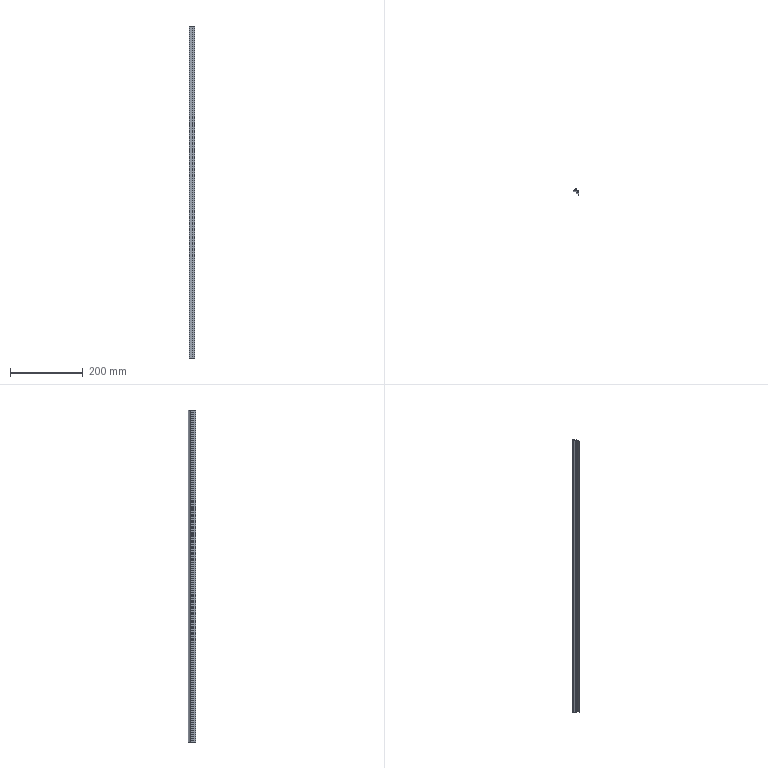Part | SolidWorks | features BaseBody 1, ICE 1, MoveFace 1 | 1 solid | 27 faces | box 14 x 20.3 x 914 mm | volume 46537 mm3 | plane 20 | cylinder 7 | commonest cylinder face diameters 0.387 x2 0.8 x2 0.4 x1 20 x1 22 x1
STEP:
#1=CARTESIAN_POINT('',(-5.304,-0.625,200.));
#2=VERTEX_POINT('',#1);
#3=CARTESIAN_POINT('',(-5.449,-0.8125,200.));
#4=VERTEX_POINT('',#3);
#5=CARTESIAN_POINT('',(-5.255,-0.8125,200.));
#6=DIRECTION('',(0.,0.,1.));
#7=DIRECTION('',(-1.,0.,0.));
#8=AXIS2_PLACEMENT_3D('',#5,#6,#7);
#9=CIRCLE('',#8,0.1937);
#10=EDGE_CURVE('',#2,#4,#9,.T.);
#11=ORIENTED_EDGE('',*,*,#10,.T.);
#12=CARTESIAN_POINT('',(-5.449,-0.8125,-714.));
#13=VERTEX_POINT('',#12);
#14=CARTESIAN_POINT('',(-5.449,-0.8125,230.));
#15=DIRECTION('',(0.,0.,-1.));
#16=VECTOR('',#15,1000.);
#17=LINE('',#14,#16);
#18=EDGE_CURVE('',#4,#13,#17,.T.);
#19=ORIENTED_EDGE('',*,*,#18,.T.);
#20=CARTESIAN_POINT('',(-5.304,-0.625,-714.));
#21=VERTEX_POINT('',#20);
#22=CARTESIAN_POINT('',(-5.255,-0.8125,-714.));
#23=DIRECTION('',(0.,0.,-1.));
#24=DIRECTION('',(1.,0.,0.));
#25=AXIS2_PLACEMENT_3D('',#22,#23,#24);
#26=CIRCLE('',#25,0.1937);
#27=EDGE_CURVE('',#13,#21,#26,.T.);
#28=ORIENTED_EDGE('',*,*,#27,.T.);
#29=CARTESIAN_POINT('',(-5.304,-0.625,230.));
#30=DIRECTION('',(0.,0.,-1.));
#31=VECTOR('',#30,1000.);
#32=LINE('',#29,#31);
#33=EDGE_CURVE('',#2,#21,#32,.T.);
#34=ORIENTED_EDGE('',*,*,#33,.F.);
#35=EDGE_LOOP('',(#11,#19,#28,#34));
#36=FACE_OUTER_BOUND('',#35,.T.);
#37=CARTESIAN_POINT('',(-5.255,-0.8125,230.));
#38=DIRECTION('',(0.,0.,-1.));
#39=DIRECTION('',(-1.,0.,0.));
#40=AXIS2_PLACEMENT_3D('',#37,#38,#39);
#41=CYLINDRICAL_SURFACE('',#40,0.1937);
#42=ADVANCED_FACE('',(#36),#41,.F.);
#43=CARTESIAN_POINT('',(5.,-1.,-714.));
#44=VERTEX_POINT('',#43);
#45=CARTESIAN_POINT('',(5.,-14.3,-714.));
#46=VERTEX_POINT('',#45);
#47=CARTESIAN_POINT('',(5.,29.623,-714.));
#48=DIRECTION('',(0.,-1.,0.));
#49=VECTOR('',#48,1000.);
#50=LINE('',#47,#49);
#51=EDGE_CURVE('',#44,#46,#50,.T.);
#52=ORIENTED_EDGE('',*,*,#51,.F.);
#53=CARTESIAN_POINT('',(5.,-1.,200.));
#54=VERTEX_POINT('',#53);
#55=CARTESIAN_POINT('',(5.,-1.,230.));
#56=DIRECTION('',(0.,0.,-1.));
#57=VECTOR('',#56,1000.);
#58=LINE('',#55,#57);
#59=EDGE_CURVE('',#54,#44,#58,.T.);
#60=ORIENTED_EDGE('',*,*,#59,.F.);
#61=CARTESIAN_POINT('',(5.,-14.3,200.));
#62=VERTEX_POINT('',#61);
#63=CARTESIAN_POINT('',(5.,-14.3,200.));
#64=DIRECTION('',(0.,1.,0.));
#65=VECTOR('',#64,1000.);
#66=LINE('',#63,#65);
#67=EDGE_CURVE('',#62,#54,#66,.T.);
#68=ORIENTED_EDGE('',*,*,#67,.F.);
#69=CARTESIAN_POINT('',(5.,-14.3,230.));
#70=DIRECTION('',(0.,0.,1.));
#71=VECTOR('',#70,1000.);
#72=LINE('',#69,#71);
#73=EDGE_CURVE('',#46,#62,#72,.T.);
#74=ORIENTED_EDGE('',*,*,#73,.F.);
#75=EDGE_LOOP('',(#52,#60,#68,#74));
#76=FACE_OUTER_BOUND('',#75,.T.);
#77=CARTESIAN_POINT('',(5.,-14.3,230.));
#78=DIRECTION('',(-1.,0.,0.));
#79=DIRECTION('',(0.,0.,1.));
#80=AXIS2_PLACEMENT_3D('',#77,#78,#79);
#81=PLANE('',#80);
#82=ADVANCED_FACE('',(#76),#81,.F.);
#83=CARTESIAN_POINT('',(-9.,-2.,-714.));
#84=VERTEX_POINT('',#83);
#85=CARTESIAN_POINT('',(-9.,-2.,200.));
#86=VERTEX_POINT('',#85);
#87=CARTESIAN_POINT('',(-9.,-2.,230.));
#88=DIRECTION('',(0.,0.,1.));
#89=VECTOR('',#88,1000.);
#90=LINE('',#87,#89);
#91=EDGE_CURVE('',#84,#86,#90,.T.);
#92=ORIENTED_EDGE('',*,*,#91,.F.);
#93=CARTESIAN_POINT('',(0.9,-2.,-714.));
#94=VERTEX_POINT('',#93);
#95=CARTESIAN_POINT('',(5.,-2.,-714.));
#96=DIRECTION('',(-1.,0.,0.));
#97=VECTOR('',#96,1000.);
#98=LINE('',#95,#97);
#99=EDGE_CURVE('',#94,#84,#98,.T.);
#100=ORIENTED_EDGE('',*,*,#99,.F.);
#101=CARTESIAN_POINT('',(0.9,-2.,200.));
#102=VERTEX_POINT('',#101);
#103=CARTESIAN_POINT('',(0.9,-2.,230.));
#104=DIRECTION('',(0.,0.,-1.));
#105=VECTOR('',#104,1000.);
#106=LINE('',#103,#105);
#107=EDGE_CURVE('',#102,#94,#106,.T.);
#108=ORIENTED_EDGE('',*,*,#107,.F.);
#109=CARTESIAN_POINT('',(5.,-2.,200.));
#110=DIRECTION('',(1.,0.,0.));
#111=VECTOR('',#110,1000.);
#112=LINE('',#109,#111);
#113=EDGE_CURVE('',#86,#102,#112,.T.);
#114=ORIENTED_EDGE('',*,*,#113,.F.);
#115=EDGE_LOOP('',(#92,#100,#108,#114));
#116=FACE_OUTER_BOUND('',#115,.T.);
#117=CARTESIAN_POINT('',(-9.,-2.,230.));
#118=DIRECTION('',(0.,1.,0.));
#119=DIRECTION('',(0.,0.,1.));
#120=AXIS2_PLACEMENT_3D('',#117,#118,#119);
#121=PLANE('',#120);
#122=ADVANCED_FACE('',(#116),#121,.F.);
#123=CARTESIAN_POINT('',(4.,-6.,200.));
#124=VERTEX_POINT('',#123);
#125=CARTESIAN_POINT('',(4.,-3.,200.));
#126=VERTEX_POINT('',#125);
#127=CARTESIAN_POINT('',(4.,29.623,200.));
#128=DIRECTION('',(0.,1.,0.));
#129=VECTOR('',#128,1000.);
#130=LINE('',#127,#129);
#131=EDGE_CURVE('',#124,#126,#130,.T.);
#132=ORIENTED_EDGE('',*,*,#131,.F.);
#133=CARTESIAN_POINT('',(1.,-6.,200.));
#134=VERTEX_POINT('',#133);
#135=CARTESIAN_POINT('',(5.,-6.,200.));
#136=DIRECTION('',(1.,0.,0.));
#137=VECTOR('',#136,1000.);
#138=LINE('',#135,#137);
#139=EDGE_CURVE('',#134,#124,#138,.T.);
#140=ORIENTED_EDGE('',*,*,#139,.F.);
#141=CARTESIAN_POINT('',(1.,-6.7,200.));
#142=VERTEX_POINT('',#141);
#143=CARTESIAN_POINT('',(1.,-6.,200.));
#144=DIRECTION('',(0.,-1.,0.));
#145=VECTOR('',#144,1000.);
#146=LINE('',#143,#145);
#147=EDGE_CURVE('',#134,#142,#146,.T.);
#148=ORIENTED_EDGE('',*,*,#147,.T.);
#149=CARTESIAN_POINT('',(-1.7,-6.7,200.));
#150=VERTEX_POINT('',#149);
#151=CARTESIAN_POINT('',(5.,-6.7,200.));
#152=DIRECTION('',(1.,0.,0.));
#153=VECTOR('',#152,1000.);
#154=LINE('',#151,#153);
#155=EDGE_CURVE('',#150,#142,#154,.T.);
#156=ORIENTED_EDGE('',*,*,#155,.F.);
#157=CARTESIAN_POINT('',(-1.7,-7.7,200.));
#158=VERTEX_POINT('',#157);
#159=CARTESIAN_POINT('',(-1.7,-6.7,200.));
#160=DIRECTION('',(0.,-1.,0.));
#161=VECTOR('',#160,1000.);
#162=LINE('',#159,#161);
#163=EDGE_CURVE('',#150,#158,#162,.T.);
#164=ORIENTED_EDGE('',*,*,#163,.T.);
#165=CARTESIAN_POINT('',(4.,-7.7,200.));
#166=VERTEX_POINT('',#165);
#167=CARTESIAN_POINT('',(5.,-7.7,200.));
#168=DIRECTION('',(-1.,0.,0.));
#169=VECTOR('',#168,1000.);
#170=LINE('',#167,#169);
#171=EDGE_CURVE('',#166,#158,#170,.T.);
#172=ORIENTED_EDGE('',*,*,#171,.F.);
#173=CARTESIAN_POINT('',(4.,-14.3,200.));
#174=VERTEX_POINT('',#173);
#175=CARTESIAN_POINT('',(4.,29.623,200.));
#176=DIRECTION('',(0.,1.,0.));
#177=VECTOR('',#176,1000.);
#178=LINE('',#175,#177);
#179=EDGE_CURVE('',#174,#166,#178,.T.);
#180=ORIENTED_EDGE('',*,*,#179,.F.);
#181=CARTESIAN_POINT('',(5.,-14.3,200.));
#182=DIRECTION('',(-1.,0.,0.));
#183=VECTOR('',#182,1000.);
#184=LINE('',#181,#183);
#185=EDGE_CURVE('',#62,#174,#184,.T.);
#186=ORIENTED_EDGE('',*,*,#185,.F.);
#187=ORIENTED_EDGE('',*,*,#67,.T.);
#188=CARTESIAN_POINT('',(-5.207,-1.,200.));
#189=VERTEX_POINT('',#188);
#190=CARTESIAN_POINT('',(5.,-1.,200.));
#191=DIRECTION('',(1.,0.,0.));
#192=VECTOR('',#191,1000.);
#193=LINE('',#190,#192);
#194=EDGE_CURVE('',#189,#54,#193,.T.);
#195=ORIENTED_EDGE('',*,*,#194,.F.);
#196=CARTESIAN_POINT('',(-5.255,-0.8125,200.));
#197=DIRECTION('',(0.,0.,1.));
#198=DIRECTION('',(-1.,0.,0.));
#199=AXIS2_PLACEMENT_3D('',#196,#197,#198);
#200=CIRCLE('',#199,0.1937);
#201=EDGE_CURVE('',#4,#189,#200,.T.);
#202=ORIENTED_EDGE('',*,*,#201,.F.);
#203=ORIENTED_EDGE('',*,*,#10,.F.);
#204=CARTESIAN_POINT('',(-1.368,3.063,200.));
#205=VERTEX_POINT('',#204);
#206=CARTESIAN_POINT('',(-10.628,9.,200.));
#207=DIRECTION('',(0.,0.,1.));
#208=DIRECTION('',(-1.,0.,0.));
#209=AXIS2_PLACEMENT_3D('',#206,#207,#208);
#210=CIRCLE('',#209,11.);
#211=EDGE_CURVE('',#2,#205,#210,.T.);
#212=ORIENTED_EDGE('',*,*,#211,.T.);
#213=CARTESIAN_POINT('',(-1.,2.955,200.));
#214=VERTEX_POINT('',#213);
#215=CARTESIAN_POINT('',(-1.2,2.955,200.));
#216=DIRECTION('',(0.,0.,1.));
#217=DIRECTION('',(-1.,0.,0.));
#218=AXIS2_PLACEMENT_3D('',#215,#216,#217);
#219=CIRCLE('',#218,0.2);
#220=EDGE_CURVE('',#214,#205,#219,.T.);
#221=ORIENTED_EDGE('',*,*,#220,.F.);
#222=CARTESIAN_POINT('',(-1.,1.5,200.));
#223=VERTEX_POINT('',#222);
#224=CARTESIAN_POINT('',(-1.,2.955,200.));
#225=DIRECTION('',(0.,1.,0.));
#226=VECTOR('',#225,1000.);
#227=LINE('',#224,#226);
#228=EDGE_CURVE('',#223,#214,#227,.T.);
#229=ORIENTED_EDGE('',*,*,#228,.F.);
#230=CARTESIAN_POINT('',(0.,1.5,200.));
#231=VERTEX_POINT('',#230);
#232=CARTESIAN_POINT('',(-1.,1.5,200.));
#233=DIRECTION('',(-1.,0.,0.));
#234=VECTOR('',#233,1000.);
#235=LINE('',#232,#234);
#236=EDGE_CURVE('',#231,#223,#235,.T.);
#237=ORIENTED_EDGE('',*,*,#236,.F.);
#238=CARTESIAN_POINT('',(0.,6.,200.));
#239=VERTEX_POINT('',#238);
#240=CARTESIAN_POINT('',(0.,1.5,200.));
#241=DIRECTION('',(0.,-1.,0.));
#242=VECTOR('',#241,1000.);
#243=LINE('',#240,#242);
#244=EDGE_CURVE('',#239,#231,#243,.T.);
#245=ORIENTED_EDGE('',*,*,#244,.F.);
#246=CARTESIAN_POINT('',(-0.8,6.,200.));
#247=VERTEX_POINT('',#246);
#248=CARTESIAN_POINT('',(0.,6.,200.));
#249=DIRECTION('',(1.,0.,0.));
#250=VECTOR('',#249,1000.);
#251=LINE('',#248,#250);
#252=EDGE_CURVE('',#247,#239,#251,.T.);
#253=ORIENTED_EDGE('',*,*,#252,.F.);
#254=CARTESIAN_POINT('',(-1.178,5.731,200.));
#255=VERTEX_POINT('',#254);
#256=CARTESIAN_POINT('',(-0.8,5.6,200.));
#257=DIRECTION('',(0.,0.,1.));
#258=DIRECTION('',(-1.,0.,0.));
#259=AXIS2_PLACEMENT_3D('',#256,#257,#258);
#260=CIRCLE('',#259,0.4);
#261=EDGE_CURVE('',#247,#255,#260,.T.);
#262=ORIENTED_EDGE('',*,*,#261,.T.);
#263=CARTESIAN_POINT('',(-8.678,-0.8077,200.));
#264=VERTEX_POINT('',#263);
#265=CARTESIAN_POINT('',(-10.628,9.,200.));
#266=DIRECTION('',(0.,0.,1.));
#267=DIRECTION('',(-1.,0.,0.));
#268=AXIS2_PLACEMENT_3D('',#265,#266,#267);
#269=CIRCLE('',#268,10.);
#270=EDGE_CURVE('',#264,#255,#269,.T.);
#271=ORIENTED_EDGE('',*,*,#270,.F.);
#272=CARTESIAN_POINT('',(-9.,-1.2,200.));
#273=VERTEX_POINT('',#272);
#274=CARTESIAN_POINT('',(-8.6,-1.2,200.));
#275=DIRECTION('',(0.,0.,1.));
#276=DIRECTION('',(-1.,0.,0.));
#277=AXIS2_PLACEMENT_3D('',#274,#275,#276);
#278=CIRCLE('',#277,0.4);
#279=EDGE_CURVE('',#264,#273,#278,.T.);
#280=ORIENTED_EDGE('',*,*,#279,.T.);
#281=CARTESIAN_POINT('',(-9.,8.,200.));
#282=DIRECTION('',(0.,-1.,0.));
#283=VECTOR('',#282,1000.);
#284=LINE('',#281,#283);
#285=EDGE_CURVE('',#273,#86,#284,.T.);
#286=ORIENTED_EDGE('',*,*,#285,.T.);
#287=ORIENTED_EDGE('',*,*,#113,.T.);
#288=CARTESIAN_POINT('',(0.9,-3.,200.));
#289=VERTEX_POINT('',#288);
#290=CARTESIAN_POINT('',(0.9,29.623,200.));
#291=DIRECTION('',(0.,1.,0.));
#292=VECTOR('',#291,1000.);
#293=LINE('',#290,#292);
#294=EDGE_CURVE('',#289,#102,#293,.T.);
#295=ORIENTED_EDGE('',*,*,#294,.F.);
#296=CARTESIAN_POINT('',(5.,-3.,200.));
#297=DIRECTION('',(-1.,0.,0.));
#298=VECTOR('',#297,1000.);
#299=LINE('',#296,#298);
#300=EDGE_CURVE('',#126,#289,#299,.T.);
#301=ORIENTED_EDGE('',*,*,#300,.F.);
#302=EDGE_LOOP('',(#132,#140,#148,#156,#164,#172,#180,#186,#187,#195,#202,#203,#212,#221,#229,#237,#245,#253,#262,#271,#280,#286,#287,#295,#301));
#303=FACE_OUTER_BOUND('',#302,.T.);
#304=CARTESIAN_POINT('',(5.,29.623,200.));
#305=DIRECTION('',(0.,0.,-1.));
#306=DIRECTION('',(-1.,0.,0.));
#307=AXIS2_PLACEMENT_3D('',#304,#305,#306);
#308=PLANE('',#307);
#309=ADVANCED_FACE('',(#303),#308,.F.);
#310=ORIENTED_EDGE('',*,*,#185,.T.);
#311=CARTESIAN_POINT('',(4.,-14.3,-714.));
#312=VERTEX_POINT('',#311);
#313=CARTESIAN_POINT('',(4.,-14.3,230.));
#314=DIRECTION('',(0.,0.,1.));
#315=VECTOR('',#314,1000.);
#316=LINE('',#313,#315);
#317=EDGE_CURVE('',#312,#174,#316,.T.);
#318=ORIENTED_EDGE('',*,*,#317,.F.);
#319=CARTESIAN_POINT('',(5.,-14.3,-714.));
#320=DIRECTION('',(-1.,0.,0.));
#321=VECTOR('',#320,1000.);
#322=LINE('',#319,#321);
#323=EDGE_CURVE('',#46,#312,#322,.T.);
#324=ORIENTED_EDGE('',*,*,#323,.F.);
#325=ORIENTED_EDGE('',*,*,#73,.T.);
#326=EDGE_LOOP('',(#310,#318,#324,#325));
#327=FACE_OUTER_BOUND('',#326,.T.);
#328=CARTESIAN_POINT('',(4.,-14.3,230.));
#329=DIRECTION('',(0.,1.,0.));
#330=DIRECTION('',(0.,0.,1.));
#331=AXIS2_PLACEMENT_3D('',#328,#329,#330);
#332=PLANE('',#331);
#333=ADVANCED_FACE('',(#327),#332,.F.);
#334=ORIENTED_EDGE('',*,*,#51,.T.);
#335=ORIENTED_EDGE('',*,*,#323,.T.);
#336=CARTESIAN_POINT('',(4.,-7.7,-714.));
#337=VERTEX_POINT('',#336);
#338=CARTESIAN_POINT('',(4.,-7.7,-714.));
#339=DIRECTION('',(0.,-1.,0.));
#340=VECTOR('',#339,1000.);
#341=LINE('',#338,#340);
#342=EDGE_CURVE('',#337,#312,#341,.T.);
#343=ORIENTED_EDGE('',*,*,#342,.F.);
#344=CARTESIAN_POINT('',(-1.7,-7.7,-714.));
#345=VERTEX_POINT('',#344);
#346=CARTESIAN_POINT('',(-1.7,-7.7,-714.));
#347=DIRECTION('',(1.,0.,0.));
#348=VECTOR('',#347,1000.);
#349=LINE('',#346,#348);
#350=EDGE_CURVE('',#345,#337,#349,.T.);
#351=ORIENTED_EDGE('',*,*,#350,.F.);
#352=CARTESIAN_POINT('',(-1.7,-6.7,-714.));
#353=VERTEX_POINT('',#352);
#354=CARTESIAN_POINT('',(-1.7,29.623,-714.));
#355=DIRECTION('',(0.,1.,0.));
#356=VECTOR('',#355,1000.);
#357=LINE('',#354,#356);
#358=EDGE_CURVE('',#345,#353,#357,.T.);
#359=ORIENTED_EDGE('',*,*,#358,.T.);
#360=CARTESIAN_POINT('',(1.,-6.7,-714.));
#361=VERTEX_POINT('',#360);
#362=CARTESIAN_POINT('',(1.,-6.7,-714.));
#363=DIRECTION('',(-1.,0.,0.));
#364=VECTOR('',#363,1000.);
#365=LINE('',#362,#364);
#366=EDGE_CURVE('',#361,#353,#365,.T.);
#367=ORIENTED_EDGE('',*,*,#366,.F.);
#368=CARTESIAN_POINT('',(1.,-6.,-714.));
#369=VERTEX_POINT('',#368);
#370=CARTESIAN_POINT('',(1.,29.623,-714.));
#371=DIRECTION('',(0.,1.,0.));
#372=VECTOR('',#371,1000.);
#373=LINE('',#370,#372);
#374=EDGE_CURVE('',#361,#369,#373,.T.);
#375=ORIENTED_EDGE('',*,*,#374,.T.);
#376=CARTESIAN_POINT('',(4.,-6.,-714.));
#377=VERTEX_POINT('',#376);
#378=CARTESIAN_POINT('',(4.,-6.,-714.));
#379=DIRECTION('',(-1.,0.,0.));
#380=VECTOR('',#379,1000.);
#381=LINE('',#378,#380);
#382=EDGE_CURVE('',#377,#369,#381,.T.);
#383=ORIENTED_EDGE('',*,*,#382,.F.);
#384=CARTESIAN_POINT('',(4.,-3.,-714.));
#385=VERTEX_POINT('',#384);
#386=CARTESIAN_POINT('',(4.,-3.,-714.));
#387=DIRECTION('',(0.,-1.,0.));
#388=VECTOR('',#387,1000.);
#389=LINE('',#386,#388);
#390=EDGE_CURVE('',#385,#377,#389,.T.);
#391=ORIENTED_EDGE('',*,*,#390,.F.);
#392=CARTESIAN_POINT('',(0.9,-3.,-714.));
#393=VERTEX_POINT('',#392);
#394=CARTESIAN_POINT('',(0.9,-3.,-714.));
#395=DIRECTION('',(1.,0.,0.));
#396=VECTOR('',#395,1000.);
#397=LINE('',#394,#396);
#398=EDGE_CURVE('',#393,#385,#397,.T.);
#399=ORIENTED_EDGE('',*,*,#398,.F.);
#400=CARTESIAN_POINT('',(0.9,-2.,-714.));
#401=DIRECTION('',(0.,-1.,0.));
#402=VECTOR('',#401,1000.);
#403=LINE('',#400,#402);
#404=EDGE_CURVE('',#94,#393,#403,.T.);
#405=ORIENTED_EDGE('',*,*,#404,.F.);
#406=ORIENTED_EDGE('',*,*,#99,.T.);
#407=CARTESIAN_POINT('',(-9.,-1.2,-714.));
#408=VERTEX_POINT('',#407);
#409=CARTESIAN_POINT('',(-9.,-1.2,-714.));
#410=DIRECTION('',(0.,-1.,0.));
#411=VECTOR('',#410,1000.);
#412=LINE('',#409,#411);
#413=EDGE_CURVE('',#408,#84,#412,.T.);
#414=ORIENTED_EDGE('',*,*,#413,.F.);
#415=CARTESIAN_POINT('',(-8.678,-0.8077,-714.));
#416=VERTEX_POINT('',#415);
#417=CARTESIAN_POINT('',(-8.6,-1.2,-714.));
#418=DIRECTION('',(0.,0.,-1.));
#419=DIRECTION('',(1.,0.,0.));
#420=AXIS2_PLACEMENT_3D('',#417,#418,#419);
#421=CIRCLE('',#420,0.4);
#422=EDGE_CURVE('',#408,#416,#421,.T.);
#423=ORIENTED_EDGE('',*,*,#422,.T.);
#424=CARTESIAN_POINT('',(-1.178,5.731,-714.));
#425=VERTEX_POINT('',#424);
#426=CARTESIAN_POINT('',(-10.628,9.,-714.));
#427=DIRECTION('',(0.,0.,-1.));
#428=DIRECTION('',(1.,0.,0.));
#429=AXIS2_PLACEMENT_3D('',#426,#427,#428);
#430=CIRCLE('',#429,10.);
#431=EDGE_CURVE('',#425,#416,#430,.T.);
#432=ORIENTED_EDGE('',*,*,#431,.F.);
#433=CARTESIAN_POINT('',(-0.8,6.,-714.));
#434=VERTEX_POINT('',#433);
#435=CARTESIAN_POINT('',(-0.8,5.6,-714.));
#436=DIRECTION('',(0.,0.,-1.));
#437=DIRECTION('',(1.,0.,0.));
#438=AXIS2_PLACEMENT_3D('',#435,#436,#437);
#439=CIRCLE('',#438,0.4);
#440=EDGE_CURVE('',#425,#434,#439,.T.);
#441=ORIENTED_EDGE('',*,*,#440,.T.);
#442=CARTESIAN_POINT('',(0.,6.,-714.));
#443=VERTEX_POINT('',#442);
#444=CARTESIAN_POINT('',(0.,6.,-714.));
#445=DIRECTION('',(-1.,0.,0.));
#446=VECTOR('',#445,1000.);
#447=LINE('',#444,#446);
#448=EDGE_CURVE('',#443,#434,#447,.T.);
#449=ORIENTED_EDGE('',*,*,#448,.F.);
#450=CARTESIAN_POINT('',(0.,1.5,-714.));
#451=VERTEX_POINT('',#450);
#452=CARTESIAN_POINT('',(0.,1.5,-714.));
#453=DIRECTION('',(0.,1.,0.));
#454=VECTOR('',#453,1000.);
#455=LINE('',#452,#454);
#456=EDGE_CURVE('',#451,#443,#455,.T.);
#457=ORIENTED_EDGE('',*,*,#456,.F.);
#458=CARTESIAN_POINT('',(-1.,1.5,-714.));
#459=VERTEX_POINT('',#458);
#460=CARTESIAN_POINT('',(-1.,1.5,-714.));
#461=DIRECTION('',(1.,0.,0.));
#462=VECTOR('',#461,1000.);
#463=LINE('',#460,#462);
#464=EDGE_CURVE('',#459,#451,#463,.T.);
#465=ORIENTED_EDGE('',*,*,#464,.F.);
#466=CARTESIAN_POINT('',(-1.,2.955,-714.));
#467=VERTEX_POINT('',#466);
#468=CARTESIAN_POINT('',(-1.,2.955,-714.));
#469=DIRECTION('',(0.,-1.,0.));
#470=VECTOR('',#469,1000.);
#471=LINE('',#468,#470);
#472=EDGE_CURVE('',#467,#459,#471,.T.);
#473=ORIENTED_EDGE('',*,*,#472,.F.);
#474=CARTESIAN_POINT('',(-1.368,3.063,-714.));
#475=VERTEX_POINT('',#474);
#476=CARTESIAN_POINT('',(-1.2,2.955,-714.));
#477=DIRECTION('',(0.,0.,-1.));
#478=DIRECTION('',(1.,0.,0.));
#479=AXIS2_PLACEMENT_3D('',#476,#477,#478);
#480=CIRCLE('',#479,0.2);
#481=EDGE_CURVE('',#475,#467,#480,.T.);
#482=ORIENTED_EDGE('',*,*,#481,.F.);
#483=CARTESIAN_POINT('',(-10.628,9.,-714.));
#484=DIRECTION('',(0.,0.,-1.));
#485=DIRECTION('',(1.,0.,0.));
#486=AXIS2_PLACEMENT_3D('',#483,#484,#485);
#487=CIRCLE('',#486,11.);
#488=EDGE_CURVE('',#475,#21,#487,.T.);
#489=ORIENTED_EDGE('',*,*,#488,.T.);
#490=ORIENTED_EDGE('',*,*,#27,.F.);
#491=CARTESIAN_POINT('',(-5.207,-1.,-714.));
#492=VERTEX_POINT('',#491);
#493=CARTESIAN_POINT('',(-5.255,-0.8125,-714.));
#494=DIRECTION('',(0.,0.,-1.));
#495=DIRECTION('',(1.,0.,0.));
#496=AXIS2_PLACEMENT_3D('',#493,#494,#495);
#497=CIRCLE('',#496,0.1937);
#498=EDGE_CURVE('',#492,#13,#497,.T.);
#499=ORIENTED_EDGE('',*,*,#498,.F.);
#500=CARTESIAN_POINT('',(5.,-1.,-714.));
#501=DIRECTION('',(-1.,0.,0.));
#502=VECTOR('',#501,1000.);
#503=LINE('',#500,#502);
#504=EDGE_CURVE('',#44,#492,#503,.T.);
#505=ORIENTED_EDGE('',*,*,#504,.F.);
#506=EDGE_LOOP('',(#334,#335,#343,#351,#359,#367,#375,#383,#391,#399,#405,#406,#414,#423,#432,#441,#449,#457,#465,#473,#482,#489,#490,#499,#505));
#507=FACE_OUTER_BOUND('',#506,.T.);
#508=CARTESIAN_POINT('',(5.,29.623,-714.));
#509=DIRECTION('',(0.,0.,1.));
#510=DIRECTION('',(1.,0.,0.));
#511=AXIS2_PLACEMENT_3D('',#508,#509,#510);
#512=PLANE('',#511);
#513=ADVANCED_FACE('',(#507),#512,.F.);
#514=ORIENTED_EDGE('',*,*,#59,.T.);
#515=ORIENTED_EDGE('',*,*,#504,.T.);
#516=CARTESIAN_POINT('',(-5.207,-1.,230.));
#517=DIRECTION('',(0.,0.,-1.));
#518=VECTOR('',#517,1000.);
#519=LINE('',#516,#518);
#520=EDGE_CURVE('',#189,#492,#519,.T.);
#521=ORIENTED_EDGE('',*,*,#520,.F.);
#522=ORIENTED_EDGE('',*,*,#194,.T.);
#523=EDGE_LOOP('',(#514,#515,#521,#522));
#524=FACE_OUTER_BOUND('',#523,.T.);
#525=CARTESIAN_POINT('',(5.,-1.,230.));
#526=DIRECTION('',(0.,-1.,0.));
#527=DIRECTION('',(0.,0.,-1.));
#528=AXIS2_PLACEMENT_3D('',#525,#526,#527);
#529=PLANE('',#528);
#530=ADVANCED_FACE('',(#524),#529,.F.);
#531=CARTESIAN_POINT('',(-9.,-1.2,230.));
#532=DIRECTION('',(0.,0.,1.));
#533=VECTOR('',#532,1000.);
#534=LINE('',#531,#533);
#535=EDGE_CURVE('',#408,#273,#534,.T.);
#536=ORIENTED_EDGE('',*,*,#535,.F.);
#537=ORIENTED_EDGE('',*,*,#413,.T.);
#538=ORIENTED_EDGE('',*,*,#91,.T.);
#539=ORIENTED_EDGE('',*,*,#285,.F.);
#540=EDGE_LOOP('',(#536,#537,#538,#539));
#541=FACE_OUTER_BOUND('',#540,.T.);
#542=CARTESIAN_POINT('',(-9.,-1.2,230.));
#543=DIRECTION('',(1.,0.,0.));
#544=DIRECTION('',(0.,0.,-1.));
#545=AXIS2_PLACEMENT_3D('',#542,#543,#544);
#546=PLANE('',#545);
#547=ADVANCED_FACE('',(#541),#546,.F.);
#548=ORIENTED_EDGE('',*,*,#294,.T.);
#549=ORIENTED_EDGE('',*,*,#107,.T.);
#550=ORIENTED_EDGE('',*,*,#404,.T.);
#551=CARTESIAN_POINT('',(0.9,-3.,230.));
#552=DIRECTION('',(0.,0.,-1.));
#553=VECTOR('',#552,1000.);
#554=LINE('',#551,#553);
#555=EDGE_CURVE('',#289,#393,#554,.T.);
#556=ORIENTED_EDGE('',*,*,#555,.F.);
#557=EDGE_LOOP('',(#548,#549,#550,#556));
#558=FACE_OUTER_BOUND('',#557,.T.);
#559=CARTESIAN_POINT('',(0.9,-2.,230.));
#560=DIRECTION('',(1.,0.,0.));
#561=DIRECTION('',(0.,0.,-1.));
#562=AXIS2_PLACEMENT_3D('',#559,#560,#561);
#563=PLANE('',#562);
#564=ADVANCED_FACE('',(#558),#563,.F.);
#565=ORIENTED_EDGE('',*,*,#300,.T.);
#566=ORIENTED_EDGE('',*,*,#555,.T.);
#567=ORIENTED_EDGE('',*,*,#398,.T.);
#568=CARTESIAN_POINT('',(4.,-3.,230.));
#569=DIRECTION('',(0.,0.,-1.));
#570=VECTOR('',#569,1000.);
#571=LINE('',#568,#570);
#572=EDGE_CURVE('',#126,#385,#571,.T.);
#573=ORIENTED_EDGE('',*,*,#572,.F.);
#574=EDGE_LOOP('',(#565,#566,#567,#573));
#575=FACE_OUTER_BOUND('',#574,.T.);
#576=CARTESIAN_POINT('',(0.9,-3.,230.));
#577=DIRECTION('',(0.,1.,0.));
#578=DIRECTION('',(0.,0.,1.));
#579=AXIS2_PLACEMENT_3D('',#576,#577,#578);
#580=PLANE('',#579);
#581=ADVANCED_FACE('',(#575),#580,.F.);
#582=ORIENTED_EDGE('',*,*,#131,.T.);
#583=ORIENTED_EDGE('',*,*,#572,.T.);
#584=ORIENTED_EDGE('',*,*,#390,.T.);
#585=CARTESIAN_POINT('',(4.,-6.,230.));
#586=DIRECTION('',(0.,0.,-1.));
#587=VECTOR('',#586,1000.);
#588=LINE('',#585,#587);
#589=EDGE_CURVE('',#124,#377,#588,.T.);
#590=ORIENTED_EDGE('',*,*,#589,.F.);
#591=EDGE_LOOP('',(#582,#583,#584,#590));
#592=FACE_OUTER_BOUND('',#591,.T.);
#593=CARTESIAN_POINT('',(4.,-3.,230.));
#594=DIRECTION('',(1.,0.,0.));
#595=DIRECTION('',(0.,0.,-1.));
#596=AXIS2_PLACEMENT_3D('',#593,#594,#595);
#597=PLANE('',#596);
#598=ADVANCED_FACE('',(#592),#597,.F.);
#599=ORIENTED_EDGE('',*,*,#139,.T.);
#600=ORIENTED_EDGE('',*,*,#589,.T.);
#601=ORIENTED_EDGE('',*,*,#382,.T.);
#602=CARTESIAN_POINT('',(1.,-6.,230.));
#603=DIRECTION('',(0.,0.,-1.));
#604=VECTOR('',#603,1000.);
#605=LINE('',#602,#604);
#606=EDGE_CURVE('',#134,#369,#605,.T.);
#607=ORIENTED_EDGE('',*,*,#606,.F.);
#608=EDGE_LOOP('',(#599,#600,#601,#607));
#609=FACE_OUTER_BOUND('',#608,.T.);
#610=CARTESIAN_POINT('',(4.,-6.,230.));
#611=DIRECTION('',(0.,-1.,0.));
#612=DIRECTION('',(0.,0.,-1.));
#613=AXIS2_PLACEMENT_3D('',#610,#611,#612);
#614=PLANE('',#613);
#615=ADVANCED_FACE('',(#609),#614,.F.);
#616=ORIENTED_EDGE('',*,*,#155,.T.);
#617=CARTESIAN_POINT('',(1.,-6.7,230.));
#618=DIRECTION('',(0.,0.,1.));
#619=VECTOR('',#618,1000.);
#620=LINE('',#617,#619);
#621=EDGE_CURVE('',#361,#142,#620,.T.);
#622=ORIENTED_EDGE('',*,*,#621,.F.);
#623=ORIENTED_EDGE('',*,*,#366,.T.);
#624=CARTESIAN_POINT('',(-1.7,-6.7,230.));
#625=DIRECTION('',(0.,0.,-1.));
#626=VECTOR('',#625,1000.);
#627=LINE('',#624,#626);
#628=EDGE_CURVE('',#150,#353,#627,.T.);
#629=ORIENTED_EDGE('',*,*,#628,.F.);
#630=EDGE_LOOP('',(#616,#622,#623,#629));
#631=FACE_OUTER_BOUND('',#630,.T.);
#632=CARTESIAN_POINT('',(1.,-6.7,230.));
#633=DIRECTION('',(0.,-1.,0.));
#634=DIRECTION('',(0.,0.,-1.));
#635=AXIS2_PLACEMENT_3D('',#632,#633,#634);
#636=PLANE('',#635);
#637=ADVANCED_FACE('',(#631),#636,.F.);
#638=ORIENTED_EDGE('',*,*,#171,.T.);
#639=CARTESIAN_POINT('',(-1.7,-7.7,230.));
#640=DIRECTION('',(0.,0.,1.));
#641=VECTOR('',#640,1000.);
#642=LINE('',#639,#641);
#643=EDGE_CURVE('',#345,#158,#642,.T.);
#644=ORIENTED_EDGE('',*,*,#643,.F.);
#645=ORIENTED_EDGE('',*,*,#350,.T.);
#646=CARTESIAN_POINT('',(4.,-7.7,230.));
#647=DIRECTION('',(0.,0.,-1.));
#648=VECTOR('',#647,1000.);
#649=LINE('',#646,#648);
#650=EDGE_CURVE('',#166,#337,#649,.T.);
#651=ORIENTED_EDGE('',*,*,#650,.F.);
#652=EDGE_LOOP('',(#638,#644,#645,#651));
#653=FACE_OUTER_BOUND('',#652,.T.);
#654=CARTESIAN_POINT('',(-1.7,-7.7,230.));
#655=DIRECTION('',(0.,1.,0.));
#656=DIRECTION('',(0.,0.,1.));
#657=AXIS2_PLACEMENT_3D('',#654,#655,#656);
#658=PLANE('',#657);
#659=ADVANCED_FACE('',(#653),#658,.F.);
#660=ORIENTED_EDGE('',*,*,#179,.T.);
#661=ORIENTED_EDGE('',*,*,#650,.T.);
#662=ORIENTED_EDGE('',*,*,#342,.T.);
#663=ORIENTED_EDGE('',*,*,#317,.T.);
#664=EDGE_LOOP('',(#660,#661,#662,#663));
#665=FACE_OUTER_BOUND('',#664,.T.);
#666=CARTESIAN_POINT('',(4.,-7.7,230.));
#667=DIRECTION('',(1.,0.,0.));
#668=DIRECTION('',(0.,0.,-1.));
#669=AXIS2_PLACEMENT_3D('',#666,#667,#668);
#670=PLANE('',#669);
#671=ADVANCED_FACE('',(#665),#670,.F.);
#672=ORIENTED_EDGE('',*,*,#18,.F.);
#673=ORIENTED_EDGE('',*,*,#201,.T.);
#674=ORIENTED_EDGE('',*,*,#520,.T.);
#675=ORIENTED_EDGE('',*,*,#498,.T.);
#676=EDGE_LOOP('',(#672,#673,#674,#675));
#677=FACE_OUTER_BOUND('',#676,.T.);
#678=CARTESIAN_POINT('',(-5.255,-0.8125,230.));
#679=DIRECTION('',(0.,0.,-1.));
#680=DIRECTION('',(-1.,0.,0.));
#681=AXIS2_PLACEMENT_3D('',#678,#679,#680);
#682=CYLINDRICAL_SURFACE('',#681,0.1937);
#683=ADVANCED_FACE('',(#677),#682,.F.);
#684=CARTESIAN_POINT('',(-1.,2.955,230.));
#685=DIRECTION('',(0.,0.,1.));
#686=VECTOR('',#685,1000.);
#687=LINE('',#684,#686);
#688=EDGE_CURVE('',#467,#214,#687,.T.);
#689=ORIENTED_EDGE('',*,*,#688,.F.);
#690=ORIENTED_EDGE('',*,*,#472,.T.);
#691=CARTESIAN_POINT('',(-1.,1.5,230.));
#692=DIRECTION('',(0.,0.,-1.));
#693=VECTOR('',#692,1000.);
#694=LINE('',#691,#693);
#695=EDGE_CURVE('',#223,#459,#694,.T.);
#696=ORIENTED_EDGE('',*,*,#695,.F.);
#697=ORIENTED_EDGE('',*,*,#228,.T.);
#698=EDGE_LOOP('',(#689,#690,#696,#697));
#699=FACE_OUTER_BOUND('',#698,.T.);
#700=CARTESIAN_POINT('',(-1.,2.955,230.));
#701=DIRECTION('',(1.,0.,0.));
#702=DIRECTION('',(0.,0.,-1.));
#703=AXIS2_PLACEMENT_3D('',#700,#701,#702);
#704=PLANE('',#703);
#705=ADVANCED_FACE('',(#699),#704,.F.);
#706=ORIENTED_EDGE('',*,*,#488,.F.);
#707=CARTESIAN_POINT('',(-1.368,3.063,230.));
#708=DIRECTION('',(0.,0.,1.));
#709=VECTOR('',#708,1000.);
#710=LINE('',#707,#709);
#711=EDGE_CURVE('',#475,#205,#710,.T.);
#712=ORIENTED_EDGE('',*,*,#711,.T.);
#713=ORIENTED_EDGE('',*,*,#211,.F.);
#714=ORIENTED_EDGE('',*,*,#33,.T.);
#715=EDGE_LOOP('',(#706,#712,#713,#714));
#716=FACE_OUTER_BOUND('',#715,.T.);
#717=CARTESIAN_POINT('',(-10.628,9.,230.));
#718=DIRECTION('',(0.,0.,-1.));
#719=DIRECTION('',(-1.,0.,0.));
#720=AXIS2_PLACEMENT_3D('',#717,#718,#719);
#721=CYLINDRICAL_SURFACE('',#720,11.);
#722=ADVANCED_FACE('',(#716),#721,.T.);
#723=CARTESIAN_POINT('',(-1.178,5.731,230.));
#724=DIRECTION('',(0.,0.,1.));
#725=VECTOR('',#724,1000.);
#726=LINE('',#723,#725);
#727=EDGE_CURVE('',#425,#255,#726,.T.);
#728=ORIENTED_EDGE('',*,*,#727,.F.);
#729=ORIENTED_EDGE('',*,*,#431,.T.);
#730=CARTESIAN_POINT('',(-8.678,-0.8077,230.));
#731=DIRECTION('',(0.,0.,-1.));
#732=VECTOR('',#731,1000.);
#733=LINE('',#730,#732);
#734=EDGE_CURVE('',#264,#416,#733,.T.);
#735=ORIENTED_EDGE('',*,*,#734,.F.);
#736=ORIENTED_EDGE('',*,*,#270,.T.);
#737=EDGE_LOOP('',(#728,#729,#735,#736));
#738=FACE_OUTER_BOUND('',#737,.T.);
#739=CARTESIAN_POINT('',(-10.628,9.,230.));
#740=DIRECTION('',(0.,0.,-1.));
#741=DIRECTION('',(-1.,0.,0.));
#742=AXIS2_PLACEMENT_3D('',#739,#740,#741);
#743=CYLINDRICAL_SURFACE('',#742,10.);
#744=ADVANCED_FACE('',(#738),#743,.F.);
#745=CARTESIAN_POINT('',(0.,1.5,230.));
#746=DIRECTION('',(0.,0.,1.));
#747=VECTOR('',#746,1000.);
#748=LINE('',#745,#747);
#749=EDGE_CURVE('',#451,#231,#748,.T.);
#750=ORIENTED_EDGE('',*,*,#749,.F.);
#751=ORIENTED_EDGE('',*,*,#456,.T.);
#752=CARTESIAN_POINT('',(0.,6.,230.));
#753=DIRECTION('',(0.,0.,-1.));
#754=VECTOR('',#753,1000.);
#755=LINE('',#752,#754);
#756=EDGE_CURVE('',#239,#443,#755,.T.);
#757=ORIENTED_EDGE('',*,*,#756,.F.);
#758=ORIENTED_EDGE('',*,*,#244,.T.);
#759=EDGE_LOOP('',(#750,#751,#757,#758));
#760=FACE_OUTER_BOUND('',#759,.T.);
#761=CARTESIAN_POINT('',(0.,1.5,230.));
#762=DIRECTION('',(-1.,0.,0.));
#763=DIRECTION('',(0.,0.,1.));
#764=AXIS2_PLACEMENT_3D('',#761,#762,#763);
#765=PLANE('',#764);
#766=ADVANCED_FACE('',(#760),#765,.F.);
#767=ORIENTED_EDGE('',*,*,#422,.F.);
#768=ORIENTED_EDGE('',*,*,#535,.T.);
#769=ORIENTED_EDGE('',*,*,#279,.F.);
#770=ORIENTED_EDGE('',*,*,#734,.T.);
#771=EDGE_LOOP('',(#767,#768,#769,#770));
#772=FACE_OUTER_BOUND('',#771,.T.);
#773=CARTESIAN_POINT('',(-8.6,-1.2,230.));
#774=DIRECTION('',(0.,0.,-1.));
#775=DIRECTION('',(-1.,0.,0.));
#776=AXIS2_PLACEMENT_3D('',#773,#774,#775);
#777=CYLINDRICAL_SURFACE('',#776,0.4);
#778=ADVANCED_FACE('',(#772),#777,.T.);
#779=ORIENTED_EDGE('',*,*,#147,.F.);
#780=ORIENTED_EDGE('',*,*,#606,.T.);
#781=ORIENTED_EDGE('',*,*,#374,.F.);
#782=ORIENTED_EDGE('',*,*,#621,.T.);
#783=EDGE_LOOP('',(#779,#780,#781,#782));
#784=FACE_OUTER_BOUND('',#783,.T.);
#785=CARTESIAN_POINT('',(1.,-6.,230.));
#786=DIRECTION('',(1.,0.,0.));
#787=DIRECTION('',(0.,0.,-1.));
#788=AXIS2_PLACEMENT_3D('',#785,#786,#787);
#789=PLANE('',#788);
#790=ADVANCED_FACE('',(#784),#789,.F.);
#791=ORIENTED_EDGE('',*,*,#163,.F.);
#792=ORIENTED_EDGE('',*,*,#628,.T.);
#793=ORIENTED_EDGE('',*,*,#358,.F.);
#794=ORIENTED_EDGE('',*,*,#643,.T.);
#795=EDGE_LOOP('',(#791,#792,#793,#794));
#796=FACE_OUTER_BOUND('',#795,.T.);
#797=CARTESIAN_POINT('',(-1.7,-6.7,230.));
#798=DIRECTION('',(1.,0.,0.));
#799=DIRECTION('',(0.,0.,-1.));
#800=AXIS2_PLACEMENT_3D('',#797,#798,#799);
#801=PLANE('',#800);
#802=ADVANCED_FACE('',(#796),#801,.F.);
#803=ORIENTED_EDGE('',*,*,#711,.F.);
#804=ORIENTED_EDGE('',*,*,#481,.T.);
#805=ORIENTED_EDGE('',*,*,#688,.T.);
#806=ORIENTED_EDGE('',*,*,#220,.T.);
#807=EDGE_LOOP('',(#803,#804,#805,#806));
#808=FACE_OUTER_BOUND('',#807,.T.);
#809=CARTESIAN_POINT('',(-1.2,2.955,230.));
#810=DIRECTION('',(0.,0.,-1.));
#811=DIRECTION('',(-1.,0.,0.));
#812=AXIS2_PLACEMENT_3D('',#809,#810,#811);
#813=CYLINDRICAL_SURFACE('',#812,0.2);
#814=ADVANCED_FACE('',(#808),#813,.F.);
#815=ORIENTED_EDGE('',*,*,#695,.T.);
#816=ORIENTED_EDGE('',*,*,#464,.T.);
#817=ORIENTED_EDGE('',*,*,#749,.T.);
#818=ORIENTED_EDGE('',*,*,#236,.T.);
#819=EDGE_LOOP('',(#815,#816,#817,#818));
#820=FACE_OUTER_BOUND('',#819,.T.);
#821=CARTESIAN_POINT('',(-1.,1.5,230.));
#822=DIRECTION('',(0.,1.,0.));
#823=DIRECTION('',(0.,0.,1.));
#824=AXIS2_PLACEMENT_3D('',#821,#822,#823);
#825=PLANE('',#824);
#826=ADVANCED_FACE('',(#820),#825,.F.);
#827=ORIENTED_EDGE('',*,*,#440,.F.);
#828=ORIENTED_EDGE('',*,*,#727,.T.);
#829=ORIENTED_EDGE('',*,*,#261,.F.);
#830=CARTESIAN_POINT('',(-0.8,6.,230.));
#831=DIRECTION('',(0.,0.,-1.));
#832=VECTOR('',#831,1000.);
#833=LINE('',#830,#832);
#834=EDGE_CURVE('',#247,#434,#833,.T.);
#835=ORIENTED_EDGE('',*,*,#834,.T.);
#836=EDGE_LOOP('',(#827,#828,#829,#835));
#837=FACE_OUTER_BOUND('',#836,.T.);
#838=CARTESIAN_POINT('',(-0.8,5.6,230.));
#839=DIRECTION('',(0.,0.,-1.));
#840=DIRECTION('',(-1.,0.,0.));
#841=AXIS2_PLACEMENT_3D('',#838,#839,#840);
#842=CYLINDRICAL_SURFACE('',#841,0.4);
#843=ADVANCED_FACE('',(#837),#842,.T.);
#844=ORIENTED_EDGE('',*,*,#756,.T.);
#845=ORIENTED_EDGE('',*,*,#448,.T.);
#846=ORIENTED_EDGE('',*,*,#834,.F.);
#847=ORIENTED_EDGE('',*,*,#252,.T.);
#848=EDGE_LOOP('',(#844,#845,#846,#847));
#849=FACE_OUTER_BOUND('',#848,.T.);
#850=CARTESIAN_POINT('',(0.,6.,230.));
#851=DIRECTION('',(0.,-1.,0.));
#852=DIRECTION('',(0.,0.,-1.));
#853=AXIS2_PLACEMENT_3D('',#850,#851,#852);
#854=PLANE('',#853);
#855=ADVANCED_FACE('',(#849),#854,.F.);
#856=CLOSED_SHELL('',(#42,#82,#122,#309,#333,#513,#530,#547,#564,#581,#598,#615,#637,#659,#671,#683,#705,#722,#744,#766,#778,#790,#802,#814,#826,#843,#855));
#857=MANIFOLD_SOLID_BREP('',#856);
#858=CARTESIAN_POINT('',(0.,0.,0.));
#859=DIRECTION('',(0.,0.,1.));
#860=DIRECTION('',(1.,0.,0.));
#861=AXIS2_PLACEMENT_3D('',#858,#859,#860);
#862=(LENGTH_UNIT()NAMED_UNIT(*)SI_UNIT(.MILLI.,.METRE.));
#863=UNCERTAINTY_MEASURE_WITH_UNIT(LENGTH_MEASURE(0.00001),#862,'','');
#864=(NAMED_UNIT(*)PLANE_ANGLE_UNIT()SI_UNIT($,.RADIAN.));
#865=(NAMED_UNIT(*)SI_UNIT($,.STERADIAN.)SOLID_ANGLE_UNIT());
#866=(GEOMETRIC_REPRESENTATION_CONTEXT(3)GLOBAL_UNCERTAINTY_ASSIGNED_CONTEXT((#863))GLOBAL_UNIT_ASSIGNED_CONTEXT((#862,#864,#865))REPRESENTATION_CONTEXT('',''));
#867=ADVANCED_BREP_SHAPE_REPRESENTATION('',(#857,#861),#866);